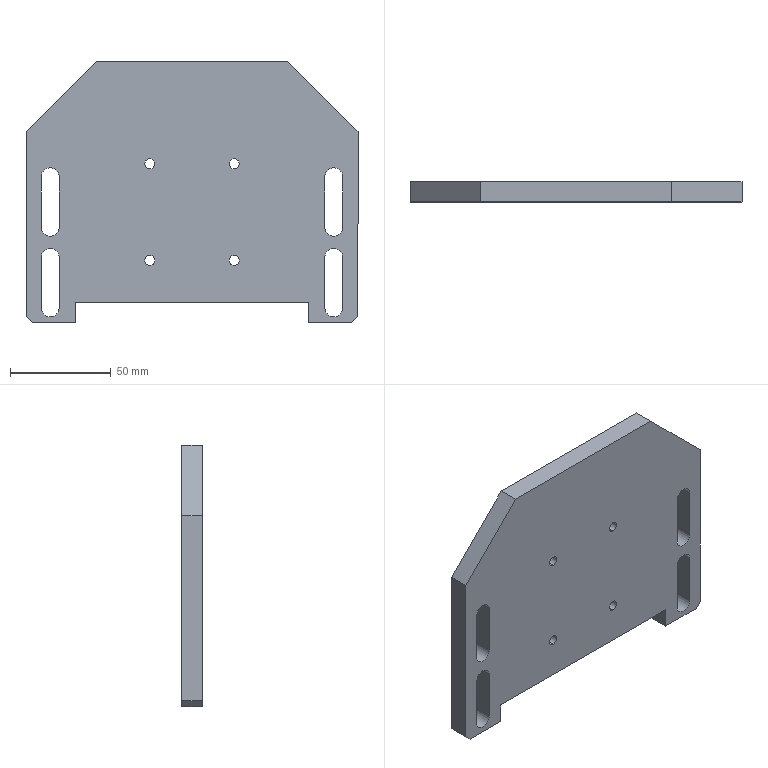Part | SolidWorks | features Chamfer 3, ICE 2, Extrusion 1, HoleWzd 1, MirrorPattern 1 | 1 solid | 42 faces | box 165 x 10 x 130 mm | volume 178230 mm3 | plane 22 | cylinder 20 | commonest cylinder face diameters 9 x12 5 x8
STEP:
#1=CARTESIAN_POINT('',(-66.,0.,7.5));
#2=VERTEX_POINT('',#1);
#3=CARTESIAN_POINT('',(-70.5,0.,12.));
#4=VERTEX_POINT('',#3);
#5=CARTESIAN_POINT('',(-70.5,0.,7.5));
#6=DIRECTION('',(0.,-1.,0.));
#7=DIRECTION('',(0.,0.,1.));
#8=AXIS2_PLACEMENT_3D('',#5,#6,#7);
#9=CIRCLE('',#8,4.5);
#10=EDGE_CURVE('',#2,#4,#9,.T.);
#11=ORIENTED_EDGE('',*,*,#10,.T.);
#12=CARTESIAN_POINT('',(-70.5,10.,12.));
#13=VERTEX_POINT('',#12);
#14=CARTESIAN_POINT('',(-70.5,0.,12.));
#15=DIRECTION('',(0.,1.,0.));
#16=VECTOR('',#15,1000.);
#17=LINE('',#14,#16);
#18=EDGE_CURVE('',#4,#13,#17,.T.);
#19=ORIENTED_EDGE('',*,*,#18,.T.);
#20=CARTESIAN_POINT('',(-66.,10.,7.5));
#21=VERTEX_POINT('',#20);
#22=CARTESIAN_POINT('',(-70.5,10.,7.5));
#23=DIRECTION('',(0.,-1.,0.));
#24=DIRECTION('',(0.,0.,1.));
#25=AXIS2_PLACEMENT_3D('',#22,#23,#24);
#26=CIRCLE('',#25,4.5);
#27=EDGE_CURVE('',#21,#13,#26,.T.);
#28=ORIENTED_EDGE('',*,*,#27,.F.);
#29=CARTESIAN_POINT('',(-66.,0.,7.5));
#30=DIRECTION('',(0.,1.,0.));
#31=VECTOR('',#30,1000.);
#32=LINE('',#29,#31);
#33=EDGE_CURVE('',#2,#21,#32,.T.);
#34=ORIENTED_EDGE('',*,*,#33,.F.);
#35=EDGE_LOOP('',(#11,#19,#28,#34));
#36=FACE_OUTER_BOUND('',#35,.T.);
#37=CARTESIAN_POINT('',(-70.5,0.,7.5));
#38=DIRECTION('',(0.,1.,0.));
#39=DIRECTION('',(0.,0.,1.));
#40=AXIS2_PLACEMENT_3D('',#37,#38,#39);
#41=CYLINDRICAL_SURFACE('',#40,4.5);
#42=ADVANCED_FACE('',(#36),#41,.F.);
#43=CARTESIAN_POINT('',(-66.,0.,-32.5));
#44=VERTEX_POINT('',#43);
#45=CARTESIAN_POINT('',(-70.5,0.,-28.));
#46=VERTEX_POINT('',#45);
#47=CARTESIAN_POINT('',(-70.5,0.,-32.5));
#48=DIRECTION('',(0.,-1.,0.));
#49=DIRECTION('',(0.,0.,1.));
#50=AXIS2_PLACEMENT_3D('',#47,#48,#49);
#51=CIRCLE('',#50,4.5);
#52=EDGE_CURVE('',#44,#46,#51,.T.);
#53=ORIENTED_EDGE('',*,*,#52,.T.);
#54=CARTESIAN_POINT('',(-70.5,10.,-28.));
#55=VERTEX_POINT('',#54);
#56=CARTESIAN_POINT('',(-70.5,0.,-28.));
#57=DIRECTION('',(0.,1.,0.));
#58=VECTOR('',#57,1000.);
#59=LINE('',#56,#58);
#60=EDGE_CURVE('',#46,#55,#59,.T.);
#61=ORIENTED_EDGE('',*,*,#60,.T.);
#62=CARTESIAN_POINT('',(-66.,10.,-32.5));
#63=VERTEX_POINT('',#62);
#64=CARTESIAN_POINT('',(-70.5,10.,-32.5));
#65=DIRECTION('',(0.,-1.,0.));
#66=DIRECTION('',(0.,0.,1.));
#67=AXIS2_PLACEMENT_3D('',#64,#65,#66);
#68=CIRCLE('',#67,4.5);
#69=EDGE_CURVE('',#63,#55,#68,.T.);
#70=ORIENTED_EDGE('',*,*,#69,.F.);
#71=CARTESIAN_POINT('',(-66.,0.,-32.5));
#72=DIRECTION('',(0.,1.,0.));
#73=VECTOR('',#72,1000.);
#74=LINE('',#71,#73);
#75=EDGE_CURVE('',#44,#63,#74,.T.);
#76=ORIENTED_EDGE('',*,*,#75,.F.);
#77=EDGE_LOOP('',(#53,#61,#70,#76));
#78=FACE_OUTER_BOUND('',#77,.T.);
#79=CARTESIAN_POINT('',(-70.5,0.,-32.5));
#80=DIRECTION('',(0.,1.,0.));
#81=DIRECTION('',(0.,0.,1.));
#82=AXIS2_PLACEMENT_3D('',#79,#80,#81);
#83=CYLINDRICAL_SURFACE('',#82,4.5);
#84=ADVANCED_FACE('',(#78),#83,.F.);
#85=CARTESIAN_POINT('',(21.,0.,11.5));
#86=VERTEX_POINT('',#85);
#87=CARTESIAN_POINT('',(21.,0.,16.5));
#88=VERTEX_POINT('',#87);
#89=CARTESIAN_POINT('',(21.,0.,14.));
#90=DIRECTION('',(0.,1.,0.));
#91=DIRECTION('',(0.,0.,1.));
#92=AXIS2_PLACEMENT_3D('',#89,#90,#91);
#93=CIRCLE('',#92,2.5);
#94=EDGE_CURVE('',#86,#88,#93,.T.);
#95=ORIENTED_EDGE('',*,*,#94,.F.);
#96=CARTESIAN_POINT('',(21.,10.,11.5));
#97=VERTEX_POINT('',#96);
#98=CARTESIAN_POINT('',(21.,10.,11.5));
#99=DIRECTION('',(0.,1.,0.));
#100=VECTOR('',#99,1000.);
#101=LINE('',#98,#100);
#102=EDGE_CURVE('',#86,#97,#101,.T.);
#103=ORIENTED_EDGE('',*,*,#102,.T.);
#104=CARTESIAN_POINT('',(21.,10.,16.5));
#105=VERTEX_POINT('',#104);
#106=CARTESIAN_POINT('',(21.,10.,14.));
#107=DIRECTION('',(0.,1.,0.));
#108=DIRECTION('',(0.,0.,1.));
#109=AXIS2_PLACEMENT_3D('',#106,#107,#108);
#110=CIRCLE('',#109,2.5);
#111=EDGE_CURVE('',#97,#105,#110,.T.);
#112=ORIENTED_EDGE('',*,*,#111,.T.);
#113=CARTESIAN_POINT('',(21.,10.,16.5));
#114=DIRECTION('',(0.,1.,0.));
#115=VECTOR('',#114,1000.);
#116=LINE('',#113,#115);
#117=EDGE_CURVE('',#88,#105,#116,.T.);
#118=ORIENTED_EDGE('',*,*,#117,.F.);
#119=EDGE_LOOP('',(#95,#103,#112,#118));
#120=FACE_OUTER_BOUND('',#119,.T.);
#121=CARTESIAN_POINT('',(21.,10.,14.));
#122=DIRECTION('',(0.,1.,0.));
#123=DIRECTION('',(0.,0.,1.));
#124=AXIS2_PLACEMENT_3D('',#121,#122,#123);
#125=CYLINDRICAL_SURFACE('',#124,2.5);
#126=ADVANCED_FACE('',(#120),#125,.F.);
#127=CARTESIAN_POINT('',(21.,0.,-36.5));
#128=VERTEX_POINT('',#127);
#129=CARTESIAN_POINT('',(21.,0.,-31.5));
#130=VERTEX_POINT('',#129);
#131=CARTESIAN_POINT('',(21.,0.,-34.));
#132=DIRECTION('',(0.,1.,0.));
#133=DIRECTION('',(0.,0.,1.));
#134=AXIS2_PLACEMENT_3D('',#131,#132,#133);
#135=CIRCLE('',#134,2.5);
#136=EDGE_CURVE('',#128,#130,#135,.T.);
#137=ORIENTED_EDGE('',*,*,#136,.F.);
#138=CARTESIAN_POINT('',(21.,10.,-36.5));
#139=VERTEX_POINT('',#138);
#140=CARTESIAN_POINT('',(21.,10.,-36.5));
#141=DIRECTION('',(0.,1.,0.));
#142=VECTOR('',#141,1000.);
#143=LINE('',#140,#142);
#144=EDGE_CURVE('',#128,#139,#143,.T.);
#145=ORIENTED_EDGE('',*,*,#144,.T.);
#146=CARTESIAN_POINT('',(21.,10.,-31.5));
#147=VERTEX_POINT('',#146);
#148=CARTESIAN_POINT('',(21.,10.,-34.));
#149=DIRECTION('',(0.,1.,0.));
#150=DIRECTION('',(0.,0.,1.));
#151=AXIS2_PLACEMENT_3D('',#148,#149,#150);
#152=CIRCLE('',#151,2.5);
#153=EDGE_CURVE('',#139,#147,#152,.T.);
#154=ORIENTED_EDGE('',*,*,#153,.T.);
#155=CARTESIAN_POINT('',(21.,10.,-31.5));
#156=DIRECTION('',(0.,1.,0.));
#157=VECTOR('',#156,1000.);
#158=LINE('',#155,#157);
#159=EDGE_CURVE('',#130,#147,#158,.T.);
#160=ORIENTED_EDGE('',*,*,#159,.F.);
#161=EDGE_LOOP('',(#137,#145,#154,#160));
#162=FACE_OUTER_BOUND('',#161,.T.);
#163=CARTESIAN_POINT('',(21.,10.,-34.));
#164=DIRECTION('',(0.,1.,0.));
#165=DIRECTION('',(0.,0.,1.));
#166=AXIS2_PLACEMENT_3D('',#163,#164,#165);
#167=CYLINDRICAL_SURFACE('',#166,2.5);
#168=ADVANCED_FACE('',(#162),#167,.F.);
#169=CARTESIAN_POINT('',(-21.,0.,-36.5));
#170=VERTEX_POINT('',#169);
#171=CARTESIAN_POINT('',(-21.,0.,-31.5));
#172=VERTEX_POINT('',#171);
#173=CARTESIAN_POINT('',(-21.,0.,-34.));
#174=DIRECTION('',(0.,1.,0.));
#175=DIRECTION('',(0.,0.,1.));
#176=AXIS2_PLACEMENT_3D('',#173,#174,#175);
#177=CIRCLE('',#176,2.5);
#178=EDGE_CURVE('',#170,#172,#177,.T.);
#179=ORIENTED_EDGE('',*,*,#178,.F.);
#180=CARTESIAN_POINT('',(-21.,10.,-36.5));
#181=VERTEX_POINT('',#180);
#182=CARTESIAN_POINT('',(-21.,10.,-36.5));
#183=DIRECTION('',(0.,1.,0.));
#184=VECTOR('',#183,1000.);
#185=LINE('',#182,#184);
#186=EDGE_CURVE('',#170,#181,#185,.T.);
#187=ORIENTED_EDGE('',*,*,#186,.T.);
#188=CARTESIAN_POINT('',(-21.,10.,-31.5));
#189=VERTEX_POINT('',#188);
#190=CARTESIAN_POINT('',(-21.,10.,-34.));
#191=DIRECTION('',(0.,1.,0.));
#192=DIRECTION('',(0.,0.,1.));
#193=AXIS2_PLACEMENT_3D('',#190,#191,#192);
#194=CIRCLE('',#193,2.5);
#195=EDGE_CURVE('',#181,#189,#194,.T.);
#196=ORIENTED_EDGE('',*,*,#195,.T.);
#197=CARTESIAN_POINT('',(-21.,10.,-31.5));
#198=DIRECTION('',(0.,1.,0.));
#199=VECTOR('',#198,1000.);
#200=LINE('',#197,#199);
#201=EDGE_CURVE('',#172,#189,#200,.T.);
#202=ORIENTED_EDGE('',*,*,#201,.F.);
#203=EDGE_LOOP('',(#179,#187,#196,#202));
#204=FACE_OUTER_BOUND('',#203,.T.);
#205=CARTESIAN_POINT('',(-21.,10.,-34.));
#206=DIRECTION('',(0.,1.,0.));
#207=DIRECTION('',(0.,0.,1.));
#208=AXIS2_PLACEMENT_3D('',#205,#206,#207);
#209=CYLINDRICAL_SURFACE('',#208,2.5);
#210=ADVANCED_FACE('',(#204),#209,.F.);
#211=CARTESIAN_POINT('',(-21.,0.,11.5));
#212=VERTEX_POINT('',#211);
#213=CARTESIAN_POINT('',(-21.,0.,16.5));
#214=VERTEX_POINT('',#213);
#215=CARTESIAN_POINT('',(-21.,0.,14.));
#216=DIRECTION('',(0.,1.,0.));
#217=DIRECTION('',(0.,0.,1.));
#218=AXIS2_PLACEMENT_3D('',#215,#216,#217);
#219=CIRCLE('',#218,2.5);
#220=EDGE_CURVE('',#212,#214,#219,.T.);
#221=ORIENTED_EDGE('',*,*,#220,.F.);
#222=CARTESIAN_POINT('',(-21.,10.,11.5));
#223=VERTEX_POINT('',#222);
#224=CARTESIAN_POINT('',(-21.,10.,11.5));
#225=DIRECTION('',(0.,1.,0.));
#226=VECTOR('',#225,1000.);
#227=LINE('',#224,#226);
#228=EDGE_CURVE('',#212,#223,#227,.T.);
#229=ORIENTED_EDGE('',*,*,#228,.T.);
#230=CARTESIAN_POINT('',(-21.,10.,16.5));
#231=VERTEX_POINT('',#230);
#232=CARTESIAN_POINT('',(-21.,10.,14.));
#233=DIRECTION('',(0.,1.,0.));
#234=DIRECTION('',(0.,0.,1.));
#235=AXIS2_PLACEMENT_3D('',#232,#233,#234);
#236=CIRCLE('',#235,2.5);
#237=EDGE_CURVE('',#223,#231,#236,.T.);
#238=ORIENTED_EDGE('',*,*,#237,.T.);
#239=CARTESIAN_POINT('',(-21.,10.,16.5));
#240=DIRECTION('',(0.,1.,0.));
#241=VECTOR('',#240,1000.);
#242=LINE('',#239,#241);
#243=EDGE_CURVE('',#214,#231,#242,.T.);
#244=ORIENTED_EDGE('',*,*,#243,.F.);
#245=EDGE_LOOP('',(#221,#229,#238,#244));
#246=FACE_OUTER_BOUND('',#245,.T.);
#247=CARTESIAN_POINT('',(-21.,10.,14.));
#248=DIRECTION('',(0.,1.,0.));
#249=DIRECTION('',(0.,0.,1.));
#250=AXIS2_PLACEMENT_3D('',#247,#248,#249);
#251=CYLINDRICAL_SURFACE('',#250,2.5);
#252=ADVANCED_FACE('',(#246),#251,.F.);
#253=CARTESIAN_POINT('',(70.5,0.,12.));
#254=VERTEX_POINT('',#253);
#255=CARTESIAN_POINT('',(75.,0.,7.5));
#256=VERTEX_POINT('',#255);
#257=CARTESIAN_POINT('',(70.5,0.,7.5));
#258=DIRECTION('',(0.,1.,0.));
#259=DIRECTION('',(0.,0.,1.));
#260=AXIS2_PLACEMENT_3D('',#257,#258,#259);
#261=CIRCLE('',#260,4.5);
#262=EDGE_CURVE('',#254,#256,#261,.T.);
#263=ORIENTED_EDGE('',*,*,#262,.F.);
#264=CARTESIAN_POINT('',(70.5,10.,12.));
#265=VERTEX_POINT('',#264);
#266=CARTESIAN_POINT('',(70.5,0.,12.));
#267=DIRECTION('',(0.,1.,0.));
#268=VECTOR('',#267,1000.);
#269=LINE('',#266,#268);
#270=EDGE_CURVE('',#254,#265,#269,.T.);
#271=ORIENTED_EDGE('',*,*,#270,.T.);
#272=CARTESIAN_POINT('',(75.,10.,7.5));
#273=VERTEX_POINT('',#272);
#274=CARTESIAN_POINT('',(70.5,10.,7.5));
#275=DIRECTION('',(0.,1.,0.));
#276=DIRECTION('',(0.,0.,1.));
#277=AXIS2_PLACEMENT_3D('',#274,#275,#276);
#278=CIRCLE('',#277,4.5);
#279=EDGE_CURVE('',#265,#273,#278,.T.);
#280=ORIENTED_EDGE('',*,*,#279,.T.);
#281=CARTESIAN_POINT('',(75.,0.,7.5));
#282=DIRECTION('',(0.,1.,0.));
#283=VECTOR('',#282,1000.);
#284=LINE('',#281,#283);
#285=EDGE_CURVE('',#256,#273,#284,.T.);
#286=ORIENTED_EDGE('',*,*,#285,.F.);
#287=EDGE_LOOP('',(#263,#271,#280,#286));
#288=FACE_OUTER_BOUND('',#287,.T.);
#289=CARTESIAN_POINT('',(70.5,0.,7.5));
#290=DIRECTION('',(0.,1.,0.));
#291=DIRECTION('',(0.,0.,1.));
#292=AXIS2_PLACEMENT_3D('',#289,#290,#291);
#293=CYLINDRICAL_SURFACE('',#292,4.5);
#294=ADVANCED_FACE('',(#288),#293,.F.);
#295=CARTESIAN_POINT('',(70.5,0.,-28.));
#296=VERTEX_POINT('',#295);
#297=CARTESIAN_POINT('',(75.,0.,-32.5));
#298=VERTEX_POINT('',#297);
#299=CARTESIAN_POINT('',(70.5,0.,-32.5));
#300=DIRECTION('',(0.,1.,0.));
#301=DIRECTION('',(0.,0.,1.));
#302=AXIS2_PLACEMENT_3D('',#299,#300,#301);
#303=CIRCLE('',#302,4.5);
#304=EDGE_CURVE('',#296,#298,#303,.T.);
#305=ORIENTED_EDGE('',*,*,#304,.F.);
#306=CARTESIAN_POINT('',(70.5,10.,-28.));
#307=VERTEX_POINT('',#306);
#308=CARTESIAN_POINT('',(70.5,0.,-28.));
#309=DIRECTION('',(0.,1.,0.));
#310=VECTOR('',#309,1000.);
#311=LINE('',#308,#310);
#312=EDGE_CURVE('',#296,#307,#311,.T.);
#313=ORIENTED_EDGE('',*,*,#312,.T.);
#314=CARTESIAN_POINT('',(75.,10.,-32.5));
#315=VERTEX_POINT('',#314);
#316=CARTESIAN_POINT('',(70.5,10.,-32.5));
#317=DIRECTION('',(0.,1.,0.));
#318=DIRECTION('',(0.,0.,1.));
#319=AXIS2_PLACEMENT_3D('',#316,#317,#318);
#320=CIRCLE('',#319,4.5);
#321=EDGE_CURVE('',#307,#315,#320,.T.);
#322=ORIENTED_EDGE('',*,*,#321,.T.);
#323=CARTESIAN_POINT('',(75.,0.,-32.5));
#324=DIRECTION('',(0.,1.,0.));
#325=VECTOR('',#324,1000.);
#326=LINE('',#323,#325);
#327=EDGE_CURVE('',#298,#315,#326,.T.);
#328=ORIENTED_EDGE('',*,*,#327,.F.);
#329=EDGE_LOOP('',(#305,#313,#322,#328));
#330=FACE_OUTER_BOUND('',#329,.T.);
#331=CARTESIAN_POINT('',(70.5,0.,-32.5));
#332=DIRECTION('',(0.,1.,0.));
#333=DIRECTION('',(0.,0.,1.));
#334=AXIS2_PLACEMENT_3D('',#331,#332,#333);
#335=CYLINDRICAL_SURFACE('',#334,4.5);
#336=ADVANCED_FACE('',(#330),#335,.F.);
#337=CARTESIAN_POINT('',(-75.,10.,-32.5));
#338=VERTEX_POINT('',#337);
#339=CARTESIAN_POINT('',(-75.,10.,-57.5));
#340=VERTEX_POINT('',#339);
#341=CARTESIAN_POINT('',(-75.,10.,-57.5));
#342=DIRECTION('',(0.,0.,-1.));
#343=VECTOR('',#342,1000.);
#344=LINE('',#341,#343);
#345=EDGE_CURVE('',#338,#340,#344,.T.);
#346=ORIENTED_EDGE('',*,*,#345,.T.);
#347=CARTESIAN_POINT('',(-66.,10.,-57.5));
#348=VERTEX_POINT('',#347);
#349=CARTESIAN_POINT('',(-70.5,10.,-57.5));
#350=DIRECTION('',(0.,-1.,0.));
#351=DIRECTION('',(0.,0.,1.));
#352=AXIS2_PLACEMENT_3D('',#349,#350,#351);
#353=CIRCLE('',#352,4.5);
#354=EDGE_CURVE('',#340,#348,#353,.T.);
#355=ORIENTED_EDGE('',*,*,#354,.T.);
#356=CARTESIAN_POINT('',(-66.,10.,-57.5));
#357=DIRECTION('',(0.,0.,1.));
#358=VECTOR('',#357,1000.);
#359=LINE('',#356,#358);
#360=EDGE_CURVE('',#348,#63,#359,.T.);
#361=ORIENTED_EDGE('',*,*,#360,.T.);
#362=ORIENTED_EDGE('',*,*,#69,.T.);
#363=CARTESIAN_POINT('',(-70.5,10.,-32.5));
#364=DIRECTION('',(0.,-1.,0.));
#365=DIRECTION('',(0.,0.,1.));
#366=AXIS2_PLACEMENT_3D('',#363,#364,#365);
#367=CIRCLE('',#366,4.5);
#368=EDGE_CURVE('',#55,#338,#367,.T.);
#369=ORIENTED_EDGE('',*,*,#368,.T.);
#370=EDGE_LOOP('',(#346,#355,#361,#362,#369));
#371=FACE_BOUND('',#370,.T.);
#372=CARTESIAN_POINT('',(21.,10.,14.));
#373=DIRECTION('',(0.,1.,0.));
#374=DIRECTION('',(0.,0.,1.));
#375=AXIS2_PLACEMENT_3D('',#372,#373,#374);
#376=CIRCLE('',#375,2.5);
#377=EDGE_CURVE('',#105,#97,#376,.T.);
#378=ORIENTED_EDGE('',*,*,#377,.F.);
#379=ORIENTED_EDGE('',*,*,#111,.F.);
#380=EDGE_LOOP('',(#378,#379));
#381=FACE_BOUND('',#380,.T.);
#382=CARTESIAN_POINT('',(21.,10.,-34.));
#383=DIRECTION('',(0.,1.,0.));
#384=DIRECTION('',(0.,0.,1.));
#385=AXIS2_PLACEMENT_3D('',#382,#383,#384);
#386=CIRCLE('',#385,2.5);
#387=EDGE_CURVE('',#147,#139,#386,.T.);
#388=ORIENTED_EDGE('',*,*,#387,.F.);
#389=ORIENTED_EDGE('',*,*,#153,.F.);
#390=EDGE_LOOP('',(#388,#389));
#391=FACE_BOUND('',#390,.T.);
#392=CARTESIAN_POINT('',(-21.,10.,-34.));
#393=DIRECTION('',(0.,1.,0.));
#394=DIRECTION('',(0.,0.,1.));
#395=AXIS2_PLACEMENT_3D('',#392,#393,#394);
#396=CIRCLE('',#395,2.5);
#397=EDGE_CURVE('',#189,#181,#396,.T.);
#398=ORIENTED_EDGE('',*,*,#397,.F.);
#399=ORIENTED_EDGE('',*,*,#195,.F.);
#400=EDGE_LOOP('',(#398,#399));
#401=FACE_BOUND('',#400,.T.);
#402=CARTESIAN_POINT('',(-21.,10.,14.));
#403=DIRECTION('',(0.,1.,0.));
#404=DIRECTION('',(0.,0.,1.));
#405=AXIS2_PLACEMENT_3D('',#402,#403,#404);
#406=CIRCLE('',#405,2.5);
#407=EDGE_CURVE('',#231,#223,#406,.T.);
#408=ORIENTED_EDGE('',*,*,#407,.F.);
#409=ORIENTED_EDGE('',*,*,#237,.F.);
#410=EDGE_LOOP('',(#408,#409));
#411=FACE_BOUND('',#410,.T.);
#412=CARTESIAN_POINT('',(75.,10.,-17.5));
#413=VERTEX_POINT('',#412);
#414=CARTESIAN_POINT('',(66.,10.,-17.5));
#415=VERTEX_POINT('',#414);
#416=CARTESIAN_POINT('',(70.5,10.,-17.5));
#417=DIRECTION('',(0.,1.,0.));
#418=DIRECTION('',(0.,0.,1.));
#419=AXIS2_PLACEMENT_3D('',#416,#417,#418);
#420=CIRCLE('',#419,4.5);
#421=EDGE_CURVE('',#413,#415,#420,.T.);
#422=ORIENTED_EDGE('',*,*,#421,.F.);
#423=CARTESIAN_POINT('',(75.,10.,-17.5));
#424=DIRECTION('',(0.,0.,-1.));
#425=VECTOR('',#424,1000.);
#426=LINE('',#423,#425);
#427=EDGE_CURVE('',#273,#413,#426,.T.);
#428=ORIENTED_EDGE('',*,*,#427,.F.);
#429=ORIENTED_EDGE('',*,*,#279,.F.);
#430=CARTESIAN_POINT('',(66.,10.,7.5));
#431=VERTEX_POINT('',#430);
#432=CARTESIAN_POINT('',(70.5,10.,7.5));
#433=DIRECTION('',(0.,1.,0.));
#434=DIRECTION('',(0.,0.,1.));
#435=AXIS2_PLACEMENT_3D('',#432,#433,#434);
#436=CIRCLE('',#435,4.5);
#437=EDGE_CURVE('',#431,#265,#436,.T.);
#438=ORIENTED_EDGE('',*,*,#437,.F.);
#439=CARTESIAN_POINT('',(66.,10.,-17.5));
#440=DIRECTION('',(0.,0.,1.));
#441=VECTOR('',#440,1000.);
#442=LINE('',#439,#441);
#443=EDGE_CURVE('',#415,#431,#442,.T.);
#444=ORIENTED_EDGE('',*,*,#443,.F.);
#445=EDGE_LOOP('',(#422,#428,#429,#438,#444));
#446=FACE_BOUND('',#445,.T.);
#447=CARTESIAN_POINT('',(75.,10.,-57.5));
#448=VERTEX_POINT('',#447);
#449=CARTESIAN_POINT('',(66.,10.,-57.5));
#450=VERTEX_POINT('',#449);
#451=CARTESIAN_POINT('',(70.5,10.,-57.5));
#452=DIRECTION('',(0.,1.,0.));
#453=DIRECTION('',(0.,0.,1.));
#454=AXIS2_PLACEMENT_3D('',#451,#452,#453);
#455=CIRCLE('',#454,4.5);
#456=EDGE_CURVE('',#448,#450,#455,.T.);
#457=ORIENTED_EDGE('',*,*,#456,.F.);
#458=CARTESIAN_POINT('',(75.,10.,-57.5));
#459=DIRECTION('',(0.,0.,-1.));
#460=VECTOR('',#459,1000.);
#461=LINE('',#458,#460);
#462=EDGE_CURVE('',#315,#448,#461,.T.);
#463=ORIENTED_EDGE('',*,*,#462,.F.);
#464=ORIENTED_EDGE('',*,*,#321,.F.);
#465=CARTESIAN_POINT('',(66.,10.,-32.5));
#466=VERTEX_POINT('',#465);
#467=CARTESIAN_POINT('',(70.5,10.,-32.5));
#468=DIRECTION('',(0.,1.,0.));
#469=DIRECTION('',(0.,0.,1.));
#470=AXIS2_PLACEMENT_3D('',#467,#468,#469);
#471=CIRCLE('',#470,4.5);
#472=EDGE_CURVE('',#466,#307,#471,.T.);
#473=ORIENTED_EDGE('',*,*,#472,.F.);
#474=CARTESIAN_POINT('',(66.,10.,-57.5));
#475=DIRECTION('',(0.,0.,1.));
#476=VECTOR('',#475,1000.);
#477=LINE('',#474,#476);
#478=EDGE_CURVE('',#450,#466,#477,.T.);
#479=ORIENTED_EDGE('',*,*,#478,.F.);
#480=EDGE_LOOP('',(#457,#463,#464,#473,#479));
#481=FACE_BOUND('',#480,.T.);
#482=CARTESIAN_POINT('',(82.5,10.,30.));
#483=VERTEX_POINT('',#482);
#484=CARTESIAN_POINT('',(82.5,10.,-62.));
#485=VERTEX_POINT('',#484);
#486=CARTESIAN_POINT('',(82.5,10.,-65.));
#487=DIRECTION('',(0.,0.,-1.));
#488=VECTOR('',#487,1000.);
#489=LINE('',#486,#488);
#490=EDGE_CURVE('',#483,#485,#489,.T.);
#491=ORIENTED_EDGE('',*,*,#490,.T.);
#492=CARTESIAN_POINT('',(79.5,10.,-65.));
#493=VERTEX_POINT('',#492);
#494=CARTESIAN_POINT('',(72.25,10.,-72.25));
#495=DIRECTION('',(-0.7071,0.,-0.7071));
#496=VECTOR('',#495,1000.);
#497=LINE('',#494,#496);
#498=EDGE_CURVE('',#485,#493,#497,.T.);
#499=ORIENTED_EDGE('',*,*,#498,.T.);
#500=CARTESIAN_POINT('',(58.,10.,-65.));
#501=VERTEX_POINT('',#500);
#502=CARTESIAN_POINT('',(-82.5,10.,-65.));
#503=DIRECTION('',(-1.,0.,0.));
#504=VECTOR('',#503,1000.);
#505=LINE('',#502,#504);
#506=EDGE_CURVE('',#493,#501,#505,.T.);
#507=ORIENTED_EDGE('',*,*,#506,.T.);
#508=CARTESIAN_POINT('',(58.,10.,-55.));
#509=VERTEX_POINT('',#508);
#510=CARTESIAN_POINT('',(58.,10.,-65.));
#511=DIRECTION('',(0.,0.,-1.));
#512=VECTOR('',#511,1000.);
#513=LINE('',#510,#512);
#514=EDGE_CURVE('',#509,#501,#513,.T.);
#515=ORIENTED_EDGE('',*,*,#514,.F.);
#516=CARTESIAN_POINT('',(-58.,10.,-55.));
#517=VERTEX_POINT('',#516);
#518=CARTESIAN_POINT('',(-58.,10.,-55.));
#519=DIRECTION('',(1.,0.,0.));
#520=VECTOR('',#519,1000.);
#521=LINE('',#518,#520);
#522=EDGE_CURVE('',#517,#509,#521,.T.);
#523=ORIENTED_EDGE('',*,*,#522,.F.);
#524=CARTESIAN_POINT('',(-58.,10.,-65.));
#525=VERTEX_POINT('',#524);
#526=CARTESIAN_POINT('',(-58.,10.,-65.));
#527=DIRECTION('',(0.,0.,1.));
#528=VECTOR('',#527,1000.);
#529=LINE('',#526,#528);
#530=EDGE_CURVE('',#525,#517,#529,.T.);
#531=ORIENTED_EDGE('',*,*,#530,.F.);
#532=CARTESIAN_POINT('',(-79.5,10.,-65.));
#533=VERTEX_POINT('',#532);
#534=CARTESIAN_POINT('',(-82.5,10.,-65.));
#535=DIRECTION('',(-1.,0.,0.));
#536=VECTOR('',#535,1000.);
#537=LINE('',#534,#536);
#538=EDGE_CURVE('',#525,#533,#537,.T.);
#539=ORIENTED_EDGE('',*,*,#538,.T.);
#540=CARTESIAN_POINT('',(-82.5,10.,-62.));
#541=VERTEX_POINT('',#540);
#542=CARTESIAN_POINT('',(-72.25,10.,-72.25));
#543=DIRECTION('',(-0.7071,0.,0.7071));
#544=VECTOR('',#543,1000.);
#545=LINE('',#542,#544);
#546=EDGE_CURVE('',#533,#541,#545,.T.);
#547=ORIENTED_EDGE('',*,*,#546,.T.);
#548=CARTESIAN_POINT('',(-82.5,10.,30.));
#549=VERTEX_POINT('',#548);
#550=CARTESIAN_POINT('',(-82.5,10.,-65.));
#551=DIRECTION('',(0.,0.,1.));
#552=VECTOR('',#551,1000.);
#553=LINE('',#550,#552);
#554=EDGE_CURVE('',#541,#549,#553,.T.);
#555=ORIENTED_EDGE('',*,*,#554,.T.);
#556=CARTESIAN_POINT('',(-47.5,10.,65.));
#557=VERTEX_POINT('',#556);
#558=CARTESIAN_POINT('',(-56.25,10.,56.25));
#559=DIRECTION('',(0.7071,0.,0.7071));
#560=VECTOR('',#559,1000.);
#561=LINE('',#558,#560);
#562=EDGE_CURVE('',#549,#557,#561,.T.);
#563=ORIENTED_EDGE('',*,*,#562,.T.);
#564=CARTESIAN_POINT('',(47.5,10.,65.));
#565=VERTEX_POINT('',#564);
#566=CARTESIAN_POINT('',(-82.5,10.,65.));
#567=DIRECTION('',(1.,0.,0.));
#568=VECTOR('',#567,1000.);
#569=LINE('',#566,#568);
#570=EDGE_CURVE('',#557,#565,#569,.T.);
#571=ORIENTED_EDGE('',*,*,#570,.T.);
#572=CARTESIAN_POINT('',(56.25,10.,56.25));
#573=DIRECTION('',(0.7071,0.,-0.7071));
#574=VECTOR('',#573,1000.);
#575=LINE('',#572,#574);
#576=EDGE_CURVE('',#565,#483,#575,.T.);
#577=ORIENTED_EDGE('',*,*,#576,.T.);
#578=EDGE_LOOP('',(#491,#499,#507,#515,#523,#531,#539,#547,#555,#563,#571,#577));
#579=FACE_OUTER_BOUND('',#578,.T.);
#580=CARTESIAN_POINT('',(-75.,10.,7.5));
#581=VERTEX_POINT('',#580);
#582=CARTESIAN_POINT('',(-75.,10.,-17.5));
#583=VERTEX_POINT('',#582);
#584=CARTESIAN_POINT('',(-75.,10.,-17.5));
#585=DIRECTION('',(0.,0.,-1.));
#586=VECTOR('',#585,1000.);
#587=LINE('',#584,#586);
#588=EDGE_CURVE('',#581,#583,#587,.T.);
#589=ORIENTED_EDGE('',*,*,#588,.T.);
#590=CARTESIAN_POINT('',(-66.,10.,-17.5));
#591=VERTEX_POINT('',#590);
#592=CARTESIAN_POINT('',(-70.5,10.,-17.5));
#593=DIRECTION('',(0.,-1.,0.));
#594=DIRECTION('',(0.,0.,1.));
#595=AXIS2_PLACEMENT_3D('',#592,#593,#594);
#596=CIRCLE('',#595,4.5);
#597=EDGE_CURVE('',#583,#591,#596,.T.);
#598=ORIENTED_EDGE('',*,*,#597,.T.);
#599=CARTESIAN_POINT('',(-66.,10.,-17.5));
#600=DIRECTION('',(0.,0.,1.));
#601=VECTOR('',#600,1000.);
#602=LINE('',#599,#601);
#603=EDGE_CURVE('',#591,#21,#602,.T.);
#604=ORIENTED_EDGE('',*,*,#603,.T.);
#605=ORIENTED_EDGE('',*,*,#27,.T.);
#606=CARTESIAN_POINT('',(-70.5,10.,7.5));
#607=DIRECTION('',(0.,-1.,0.));
#608=DIRECTION('',(0.,0.,1.));
#609=AXIS2_PLACEMENT_3D('',#606,#607,#608);
#610=CIRCLE('',#609,4.5);
#611=EDGE_CURVE('',#13,#581,#610,.T.);
#612=ORIENTED_EDGE('',*,*,#611,.T.);
#613=EDGE_LOOP('',(#589,#598,#604,#605,#612));
#614=FACE_BOUND('',#613,.T.);
#615=CARTESIAN_POINT('',(0.,10.,0.));
#616=DIRECTION('',(0.,1.,0.));
#617=DIRECTION('',(0.,0.,1.));
#618=AXIS2_PLACEMENT_3D('',#615,#616,#617);
#619=PLANE('',#618);
#620=ADVANCED_FACE('',(#371,#381,#391,#401,#411,#446,#481,#579,#614),#619,.T.);
#621=CARTESIAN_POINT('',(-75.,0.,-57.5));
#622=VERTEX_POINT('',#621);
#623=CARTESIAN_POINT('',(-66.,0.,-57.5));
#624=VERTEX_POINT('',#623);
#625=CARTESIAN_POINT('',(-70.5,0.,-57.5));
#626=DIRECTION('',(0.,-1.,0.));
#627=DIRECTION('',(0.,0.,1.));
#628=AXIS2_PLACEMENT_3D('',#625,#626,#627);
#629=CIRCLE('',#628,4.5);
#630=EDGE_CURVE('',#622,#624,#629,.T.);
#631=ORIENTED_EDGE('',*,*,#630,.F.);
#632=CARTESIAN_POINT('',(-75.,0.,-32.5));
#633=VERTEX_POINT('',#632);
#634=CARTESIAN_POINT('',(-75.,0.,-57.5));
#635=DIRECTION('',(0.,0.,-1.));
#636=VECTOR('',#635,1000.);
#637=LINE('',#634,#636);
#638=EDGE_CURVE('',#633,#622,#637,.T.);
#639=ORIENTED_EDGE('',*,*,#638,.F.);
#640=CARTESIAN_POINT('',(-70.5,0.,-32.5));
#641=DIRECTION('',(0.,-1.,0.));
#642=DIRECTION('',(0.,0.,1.));
#643=AXIS2_PLACEMENT_3D('',#640,#641,#642);
#644=CIRCLE('',#643,4.5);
#645=EDGE_CURVE('',#46,#633,#644,.T.);
#646=ORIENTED_EDGE('',*,*,#645,.F.);
#647=ORIENTED_EDGE('',*,*,#52,.F.);
#648=CARTESIAN_POINT('',(-66.,0.,-57.5));
#649=DIRECTION('',(0.,0.,1.));
#650=VECTOR('',#649,1000.);
#651=LINE('',#648,#650);
#652=EDGE_CURVE('',#624,#44,#651,.T.);
#653=ORIENTED_EDGE('',*,*,#652,.F.);
#654=EDGE_LOOP('',(#631,#639,#646,#647,#653));
#655=FACE_BOUND('',#654,.T.);
#656=CARTESIAN_POINT('',(21.,0.,14.));
#657=DIRECTION('',(0.,1.,0.));
#658=DIRECTION('',(0.,0.,1.));
#659=AXIS2_PLACEMENT_3D('',#656,#657,#658);
#660=CIRCLE('',#659,2.5);
#661=EDGE_CURVE('',#88,#86,#660,.T.);
#662=ORIENTED_EDGE('',*,*,#661,.T.);
#663=ORIENTED_EDGE('',*,*,#94,.T.);
#664=EDGE_LOOP('',(#662,#663));
#665=FACE_BOUND('',#664,.T.);
#666=CARTESIAN_POINT('',(21.,0.,-34.));
#667=DIRECTION('',(0.,1.,0.));
#668=DIRECTION('',(0.,0.,1.));
#669=AXIS2_PLACEMENT_3D('',#666,#667,#668);
#670=CIRCLE('',#669,2.5);
#671=EDGE_CURVE('',#130,#128,#670,.T.);
#672=ORIENTED_EDGE('',*,*,#671,.T.);
#673=ORIENTED_EDGE('',*,*,#136,.T.);
#674=EDGE_LOOP('',(#672,#673));
#675=FACE_BOUND('',#674,.T.);
#676=CARTESIAN_POINT('',(-21.,0.,-34.));
#677=DIRECTION('',(0.,1.,0.));
#678=DIRECTION('',(0.,0.,1.));
#679=AXIS2_PLACEMENT_3D('',#676,#677,#678);
#680=CIRCLE('',#679,2.5);
#681=EDGE_CURVE('',#172,#170,#680,.T.);
#682=ORIENTED_EDGE('',*,*,#681,.T.);
#683=ORIENTED_EDGE('',*,*,#178,.T.);
#684=EDGE_LOOP('',(#682,#683));
#685=FACE_BOUND('',#684,.T.);
#686=CARTESIAN_POINT('',(-21.,0.,14.));
#687=DIRECTION('',(0.,1.,0.));
#688=DIRECTION('',(0.,0.,1.));
#689=AXIS2_PLACEMENT_3D('',#686,#687,#688);
#690=CIRCLE('',#689,2.5);
#691=EDGE_CURVE('',#214,#212,#690,.T.);
#692=ORIENTED_EDGE('',*,*,#691,.T.);
#693=ORIENTED_EDGE('',*,*,#220,.T.);
#694=EDGE_LOOP('',(#692,#693));
#695=FACE_BOUND('',#694,.T.);
#696=CARTESIAN_POINT('',(75.,0.,-17.5));
#697=VERTEX_POINT('',#696);
#698=CARTESIAN_POINT('',(75.,0.,-17.5));
#699=DIRECTION('',(0.,0.,-1.));
#700=VECTOR('',#699,1000.);
#701=LINE('',#698,#700);
#702=EDGE_CURVE('',#256,#697,#701,.T.);
#703=ORIENTED_EDGE('',*,*,#702,.T.);
#704=CARTESIAN_POINT('',(66.,0.,-17.5));
#705=VERTEX_POINT('',#704);
#706=CARTESIAN_POINT('',(70.5,0.,-17.5));
#707=DIRECTION('',(0.,1.,0.));
#708=DIRECTION('',(0.,0.,1.));
#709=AXIS2_PLACEMENT_3D('',#706,#707,#708);
#710=CIRCLE('',#709,4.5);
#711=EDGE_CURVE('',#697,#705,#710,.T.);
#712=ORIENTED_EDGE('',*,*,#711,.T.);
#713=CARTESIAN_POINT('',(66.,0.,7.5));
#714=VERTEX_POINT('',#713);
#715=CARTESIAN_POINT('',(66.,0.,-17.5));
#716=DIRECTION('',(0.,0.,1.));
#717=VECTOR('',#716,1000.);
#718=LINE('',#715,#717);
#719=EDGE_CURVE('',#705,#714,#718,.T.);
#720=ORIENTED_EDGE('',*,*,#719,.T.);
#721=CARTESIAN_POINT('',(70.5,0.,7.5));
#722=DIRECTION('',(0.,1.,0.));
#723=DIRECTION('',(0.,0.,1.));
#724=AXIS2_PLACEMENT_3D('',#721,#722,#723);
#725=CIRCLE('',#724,4.5);
#726=EDGE_CURVE('',#714,#254,#725,.T.);
#727=ORIENTED_EDGE('',*,*,#726,.T.);
#728=ORIENTED_EDGE('',*,*,#262,.T.);
#729=EDGE_LOOP('',(#703,#712,#720,#727,#728));
#730=FACE_BOUND('',#729,.T.);
#731=CARTESIAN_POINT('',(75.,0.,-57.5));
#732=VERTEX_POINT('',#731);
#733=CARTESIAN_POINT('',(75.,0.,-57.5));
#734=DIRECTION('',(0.,0.,-1.));
#735=VECTOR('',#734,1000.);
#736=LINE('',#733,#735);
#737=EDGE_CURVE('',#298,#732,#736,.T.);
#738=ORIENTED_EDGE('',*,*,#737,.T.);
#739=CARTESIAN_POINT('',(66.,0.,-57.5));
#740=VERTEX_POINT('',#739);
#741=CARTESIAN_POINT('',(70.5,0.,-57.5));
#742=DIRECTION('',(0.,1.,0.));
#743=DIRECTION('',(0.,0.,1.));
#744=AXIS2_PLACEMENT_3D('',#741,#742,#743);
#745=CIRCLE('',#744,4.5);
#746=EDGE_CURVE('',#732,#740,#745,.T.);
#747=ORIENTED_EDGE('',*,*,#746,.T.);
#748=CARTESIAN_POINT('',(66.,0.,-32.5));
#749=VERTEX_POINT('',#748);
#750=CARTESIAN_POINT('',(66.,0.,-57.5));
#751=DIRECTION('',(0.,0.,1.));
#752=VECTOR('',#751,1000.);
#753=LINE('',#750,#752);
#754=EDGE_CURVE('',#740,#749,#753,.T.);
#755=ORIENTED_EDGE('',*,*,#754,.T.);
#756=CARTESIAN_POINT('',(70.5,0.,-32.5));
#757=DIRECTION('',(0.,1.,0.));
#758=DIRECTION('',(0.,0.,1.));
#759=AXIS2_PLACEMENT_3D('',#756,#757,#758);
#760=CIRCLE('',#759,4.5);
#761=EDGE_CURVE('',#749,#296,#760,.T.);
#762=ORIENTED_EDGE('',*,*,#761,.T.);
#763=ORIENTED_EDGE('',*,*,#304,.T.);
#764=EDGE_LOOP('',(#738,#747,#755,#762,#763));
#765=FACE_BOUND('',#764,.T.);
#766=CARTESIAN_POINT('',(79.5,0.,-65.));
#767=VERTEX_POINT('',#766);
#768=CARTESIAN_POINT('',(58.,0.,-65.));
#769=VERTEX_POINT('',#768);
#770=CARTESIAN_POINT('',(-82.5,0.,-65.));
#771=DIRECTION('',(-1.,0.,0.));
#772=VECTOR('',#771,1000.);
#773=LINE('',#770,#772);
#774=EDGE_CURVE('',#767,#769,#773,.T.);
#775=ORIENTED_EDGE('',*,*,#774,.F.);
#776=CARTESIAN_POINT('',(82.5,0.,-62.));
#777=VERTEX_POINT('',#776);
#778=CARTESIAN_POINT('',(79.5,0.,-65.));
#779=DIRECTION('',(0.7071,0.,0.7071));
#780=VECTOR('',#779,1000.);
#781=LINE('',#778,#780);
#782=EDGE_CURVE('',#767,#777,#781,.T.);
#783=ORIENTED_EDGE('',*,*,#782,.T.);
#784=CARTESIAN_POINT('',(82.5,0.,30.));
#785=VERTEX_POINT('',#784);
#786=CARTESIAN_POINT('',(82.5,0.,-65.));
#787=DIRECTION('',(0.,0.,-1.));
#788=VECTOR('',#787,1000.);
#789=LINE('',#786,#788);
#790=EDGE_CURVE('',#785,#777,#789,.T.);
#791=ORIENTED_EDGE('',*,*,#790,.F.);
#792=CARTESIAN_POINT('',(47.5,0.,65.));
#793=VERTEX_POINT('',#792);
#794=CARTESIAN_POINT('',(82.5,0.,30.));
#795=DIRECTION('',(-0.7071,0.,0.7071));
#796=VECTOR('',#795,1000.);
#797=LINE('',#794,#796);
#798=EDGE_CURVE('',#785,#793,#797,.T.);
#799=ORIENTED_EDGE('',*,*,#798,.T.);
#800=CARTESIAN_POINT('',(-47.5,0.,65.));
#801=VERTEX_POINT('',#800);
#802=CARTESIAN_POINT('',(-82.5,0.,65.));
#803=DIRECTION('',(1.,0.,0.));
#804=VECTOR('',#803,1000.);
#805=LINE('',#802,#804);
#806=EDGE_CURVE('',#801,#793,#805,.T.);
#807=ORIENTED_EDGE('',*,*,#806,.F.);
#808=CARTESIAN_POINT('',(-82.5,0.,30.));
#809=VERTEX_POINT('',#808);
#810=CARTESIAN_POINT('',(-47.5,0.,65.));
#811=DIRECTION('',(-0.7071,0.,-0.7071));
#812=VECTOR('',#811,1000.);
#813=LINE('',#810,#812);
#814=EDGE_CURVE('',#801,#809,#813,.T.);
#815=ORIENTED_EDGE('',*,*,#814,.T.);
#816=CARTESIAN_POINT('',(-82.5,0.,-62.));
#817=VERTEX_POINT('',#816);
#818=CARTESIAN_POINT('',(-82.5,0.,-65.));
#819=DIRECTION('',(0.,0.,1.));
#820=VECTOR('',#819,1000.);
#821=LINE('',#818,#820);
#822=EDGE_CURVE('',#817,#809,#821,.T.);
#823=ORIENTED_EDGE('',*,*,#822,.F.);
#824=CARTESIAN_POINT('',(-79.5,0.,-65.));
#825=VERTEX_POINT('',#824);
#826=CARTESIAN_POINT('',(-82.5,0.,-62.));
#827=DIRECTION('',(0.7071,0.,-0.7071));
#828=VECTOR('',#827,1000.);
#829=LINE('',#826,#828);
#830=EDGE_CURVE('',#817,#825,#829,.T.);
#831=ORIENTED_EDGE('',*,*,#830,.T.);
#832=CARTESIAN_POINT('',(-58.,0.,-65.));
#833=VERTEX_POINT('',#832);
#834=CARTESIAN_POINT('',(-82.5,0.,-65.));
#835=DIRECTION('',(-1.,0.,0.));
#836=VECTOR('',#835,1000.);
#837=LINE('',#834,#836);
#838=EDGE_CURVE('',#833,#825,#837,.T.);
#839=ORIENTED_EDGE('',*,*,#838,.F.);
#840=CARTESIAN_POINT('',(-58.,0.,-55.));
#841=VERTEX_POINT('',#840);
#842=CARTESIAN_POINT('',(-58.,0.,-65.));
#843=DIRECTION('',(0.,0.,1.));
#844=VECTOR('',#843,1000.);
#845=LINE('',#842,#844);
#846=EDGE_CURVE('',#833,#841,#845,.T.);
#847=ORIENTED_EDGE('',*,*,#846,.T.);
#848=CARTESIAN_POINT('',(58.,0.,-55.));
#849=VERTEX_POINT('',#848);
#850=CARTESIAN_POINT('',(-58.,0.,-55.));
#851=DIRECTION('',(1.,0.,0.));
#852=VECTOR('',#851,1000.);
#853=LINE('',#850,#852);
#854=EDGE_CURVE('',#841,#849,#853,.T.);
#855=ORIENTED_EDGE('',*,*,#854,.T.);
#856=CARTESIAN_POINT('',(58.,0.,-65.));
#857=DIRECTION('',(0.,0.,-1.));
#858=VECTOR('',#857,1000.);
#859=LINE('',#856,#858);
#860=EDGE_CURVE('',#849,#769,#859,.T.);
#861=ORIENTED_EDGE('',*,*,#860,.T.);
#862=EDGE_LOOP('',(#775,#783,#791,#799,#807,#815,#823,#831,#839,#847,#855,#861));
#863=FACE_OUTER_BOUND('',#862,.T.);
#864=CARTESIAN_POINT('',(-75.,0.,-17.5));
#865=VERTEX_POINT('',#864);
#866=CARTESIAN_POINT('',(-66.,0.,-17.5));
#867=VERTEX_POINT('',#866);
#868=CARTESIAN_POINT('',(-70.5,0.,-17.5));
#869=DIRECTION('',(0.,-1.,0.));
#870=DIRECTION('',(0.,0.,1.));
#871=AXIS2_PLACEMENT_3D('',#868,#869,#870);
#872=CIRCLE('',#871,4.5);
#873=EDGE_CURVE('',#865,#867,#872,.T.);
#874=ORIENTED_EDGE('',*,*,#873,.F.);
#875=CARTESIAN_POINT('',(-75.,0.,7.5));
#876=VERTEX_POINT('',#875);
#877=CARTESIAN_POINT('',(-75.,0.,-17.5));
#878=DIRECTION('',(0.,0.,-1.));
#879=VECTOR('',#878,1000.);
#880=LINE('',#877,#879);
#881=EDGE_CURVE('',#876,#865,#880,.T.);
#882=ORIENTED_EDGE('',*,*,#881,.F.);
#883=CARTESIAN_POINT('',(-70.5,0.,7.5));
#884=DIRECTION('',(0.,-1.,0.));
#885=DIRECTION('',(0.,0.,1.));
#886=AXIS2_PLACEMENT_3D('',#883,#884,#885);
#887=CIRCLE('',#886,4.5);
#888=EDGE_CURVE('',#4,#876,#887,.T.);
#889=ORIENTED_EDGE('',*,*,#888,.F.);
#890=ORIENTED_EDGE('',*,*,#10,.F.);
#891=CARTESIAN_POINT('',(-66.,0.,-17.5));
#892=DIRECTION('',(0.,0.,1.));
#893=VECTOR('',#892,1000.);
#894=LINE('',#891,#893);
#895=EDGE_CURVE('',#867,#2,#894,.T.);
#896=ORIENTED_EDGE('',*,*,#895,.F.);
#897=EDGE_LOOP('',(#874,#882,#889,#890,#896));
#898=FACE_BOUND('',#897,.T.);
#899=CARTESIAN_POINT('',(0.,0.,0.));
#900=DIRECTION('',(0.,1.,0.));
#901=DIRECTION('',(0.,0.,1.));
#902=AXIS2_PLACEMENT_3D('',#899,#900,#901);
#903=PLANE('',#902);
#904=ADVANCED_FACE('',(#655,#665,#675,#685,#695,#730,#765,#863,#898),#903,.F.);
#905=ORIENTED_EDGE('',*,*,#838,.T.);
#906=CARTESIAN_POINT('',(-79.5,10.,-65.));
#907=DIRECTION('',(0.,1.,0.));
#908=VECTOR('',#907,1000.);
#909=LINE('',#906,#908);
#910=EDGE_CURVE('',#825,#533,#909,.T.);
#911=ORIENTED_EDGE('',*,*,#910,.T.);
#912=ORIENTED_EDGE('',*,*,#538,.F.);
#913=CARTESIAN_POINT('',(-58.,0.,-65.));
#914=DIRECTION('',(0.,1.,0.));
#915=VECTOR('',#914,1000.);
#916=LINE('',#913,#915);
#917=EDGE_CURVE('',#833,#525,#916,.T.);
#918=ORIENTED_EDGE('',*,*,#917,.F.);
#919=EDGE_LOOP('',(#905,#911,#912,#918));
#920=FACE_OUTER_BOUND('',#919,.T.);
#921=CARTESIAN_POINT('',(-82.5,10.,-65.));
#922=DIRECTION('',(0.,0.,1.));
#923=DIRECTION('',(1.,0.,0.));
#924=AXIS2_PLACEMENT_3D('',#921,#922,#923);
#925=PLANE('',#924);
#926=ADVANCED_FACE('',(#920),#925,.F.);
#927=ORIENTED_EDGE('',*,*,#790,.T.);
#928=CARTESIAN_POINT('',(82.5,10.,-62.));
#929=DIRECTION('',(0.,1.,0.));
#930=VECTOR('',#929,1000.);
#931=LINE('',#928,#930);
#932=EDGE_CURVE('',#777,#485,#931,.T.);
#933=ORIENTED_EDGE('',*,*,#932,.T.);
#934=ORIENTED_EDGE('',*,*,#490,.F.);
#935=CARTESIAN_POINT('',(82.5,10.,30.));
#936=DIRECTION('',(0.,-1.,0.));
#937=VECTOR('',#936,1000.);
#938=LINE('',#935,#937);
#939=EDGE_CURVE('',#483,#785,#938,.T.);
#940=ORIENTED_EDGE('',*,*,#939,.T.);
#941=EDGE_LOOP('',(#927,#933,#934,#940));
#942=FACE_OUTER_BOUND('',#941,.T.);
#943=CARTESIAN_POINT('',(82.5,10.,-65.));
#944=DIRECTION('',(-1.,0.,0.));
#945=DIRECTION('',(0.,0.,1.));
#946=AXIS2_PLACEMENT_3D('',#943,#944,#945);
#947=PLANE('',#946);
#948=ADVANCED_FACE('',(#942),#947,.F.);
#949=ORIENTED_EDGE('',*,*,#506,.F.);
#950=CARTESIAN_POINT('',(79.5,10.,-65.));
#951=DIRECTION('',(0.,-1.,0.));
#952=VECTOR('',#951,1000.);
#953=LINE('',#950,#952);
#954=EDGE_CURVE('',#493,#767,#953,.T.);
#955=ORIENTED_EDGE('',*,*,#954,.T.);
#956=ORIENTED_EDGE('',*,*,#774,.T.);
#957=CARTESIAN_POINT('',(58.,0.,-65.));
#958=DIRECTION('',(0.,1.,0.));
#959=VECTOR('',#958,1000.);
#960=LINE('',#957,#959);
#961=EDGE_CURVE('',#769,#501,#960,.T.);
#962=ORIENTED_EDGE('',*,*,#961,.T.);
#963=EDGE_LOOP('',(#949,#955,#956,#962));
#964=FACE_OUTER_BOUND('',#963,.T.);
#965=CARTESIAN_POINT('',(-82.5,10.,-65.));
#966=DIRECTION('',(0.,0.,1.));
#967=DIRECTION('',(1.,0.,0.));
#968=AXIS2_PLACEMENT_3D('',#965,#966,#967);
#969=PLANE('',#968);
#970=ADVANCED_FACE('',(#964),#969,.F.);
#971=ORIENTED_EDGE('',*,*,#554,.F.);
#972=CARTESIAN_POINT('',(-82.5,10.,-62.));
#973=DIRECTION('',(0.,-1.,0.));
#974=VECTOR('',#973,1000.);
#975=LINE('',#972,#974);
#976=EDGE_CURVE('',#541,#817,#975,.T.);
#977=ORIENTED_EDGE('',*,*,#976,.T.);
#978=ORIENTED_EDGE('',*,*,#822,.T.);
#979=CARTESIAN_POINT('',(-82.5,10.,30.));
#980=DIRECTION('',(0.,1.,0.));
#981=VECTOR('',#980,1000.);
#982=LINE('',#979,#981);
#983=EDGE_CURVE('',#809,#549,#982,.T.);
#984=ORIENTED_EDGE('',*,*,#983,.T.);
#985=EDGE_LOOP('',(#971,#977,#978,#984));
#986=FACE_OUTER_BOUND('',#985,.T.);
#987=CARTESIAN_POINT('',(-82.5,10.,-65.));
#988=DIRECTION('',(1.,0.,0.));
#989=DIRECTION('',(0.,0.,-1.));
#990=AXIS2_PLACEMENT_3D('',#987,#988,#989);
#991=PLANE('',#990);
#992=ADVANCED_FACE('',(#986),#991,.F.);
#993=ORIENTED_EDGE('',*,*,#806,.T.);
#994=CARTESIAN_POINT('',(47.5,10.,65.));
#995=DIRECTION('',(0.,1.,0.));
#996=VECTOR('',#995,1000.);
#997=LINE('',#994,#996);
#998=EDGE_CURVE('',#793,#565,#997,.T.);
#999=ORIENTED_EDGE('',*,*,#998,.T.);
#1000=ORIENTED_EDGE('',*,*,#570,.F.);
#1001=CARTESIAN_POINT('',(-47.5,10.,65.));
#1002=DIRECTION('',(0.,-1.,0.));
#1003=VECTOR('',#1002,1000.);
#1004=LINE('',#1001,#1003);
#1005=EDGE_CURVE('',#557,#801,#1004,.T.);
#1006=ORIENTED_EDGE('',*,*,#1005,.T.);
#1007=EDGE_LOOP('',(#993,#999,#1000,#1006));
#1008=FACE_OUTER_BOUND('',#1007,.T.);
#1009=CARTESIAN_POINT('',(-82.5,10.,65.));
#1010=DIRECTION('',(0.,0.,-1.));
#1011=DIRECTION('',(-1.,0.,0.));
#1012=AXIS2_PLACEMENT_3D('',#1009,#1010,#1011);
#1013=PLANE('',#1012);
#1014=ADVANCED_FACE('',(#1008),#1013,.F.);
#1015=ORIENTED_EDGE('',*,*,#530,.T.);
#1016=CARTESIAN_POINT('',(-58.,0.,-55.));
#1017=DIRECTION('',(0.,1.,0.));
#1018=VECTOR('',#1017,1000.);
#1019=LINE('',#1016,#1018);
#1020=EDGE_CURVE('',#841,#517,#1019,.T.);
#1021=ORIENTED_EDGE('',*,*,#1020,.F.);
#1022=ORIENTED_EDGE('',*,*,#846,.F.);
#1023=ORIENTED_EDGE('',*,*,#917,.T.);
#1024=EDGE_LOOP('',(#1015,#1021,#1022,#1023));
#1025=FACE_OUTER_BOUND('',#1024,.T.);
#1026=CARTESIAN_POINT('',(-58.,0.,-65.));
#1027=DIRECTION('',(-1.,0.,0.));
#1028=DIRECTION('',(0.,0.,1.));
#1029=AXIS2_PLACEMENT_3D('',#1026,#1027,#1028);
#1030=PLANE('',#1029);
#1031=ADVANCED_FACE('',(#1025),#1030,.F.);
#1032=ORIENTED_EDGE('',*,*,#514,.T.);
#1033=ORIENTED_EDGE('',*,*,#961,.F.);
#1034=ORIENTED_EDGE('',*,*,#860,.F.);
#1035=CARTESIAN_POINT('',(58.,0.,-55.));
#1036=DIRECTION('',(0.,1.,0.));
#1037=VECTOR('',#1036,1000.);
#1038=LINE('',#1035,#1037);
#1039=EDGE_CURVE('',#849,#509,#1038,.T.);
#1040=ORIENTED_EDGE('',*,*,#1039,.T.);
#1041=EDGE_LOOP('',(#1032,#1033,#1034,#1040));
#1042=FACE_OUTER_BOUND('',#1041,.T.);
#1043=CARTESIAN_POINT('',(58.,0.,-65.));
#1044=DIRECTION('',(1.,0.,0.));
#1045=DIRECTION('',(0.,0.,-1.));
#1046=AXIS2_PLACEMENT_3D('',#1043,#1044,#1045);
#1047=PLANE('',#1046);
#1048=ADVANCED_FACE('',(#1042),#1047,.F.);
#1049=ORIENTED_EDGE('',*,*,#522,.T.);
#1050=ORIENTED_EDGE('',*,*,#1039,.F.);
#1051=ORIENTED_EDGE('',*,*,#854,.F.);
#1052=ORIENTED_EDGE('',*,*,#1020,.T.);
#1053=EDGE_LOOP('',(#1049,#1050,#1051,#1052));
#1054=FACE_OUTER_BOUND('',#1053,.T.);
#1055=CARTESIAN_POINT('',(-58.,0.,-55.));
#1056=DIRECTION('',(0.,0.,1.));
#1057=DIRECTION('',(1.,0.,0.));
#1058=AXIS2_PLACEMENT_3D('',#1055,#1056,#1057);
#1059=PLANE('',#1058);
#1060=ADVANCED_FACE('',(#1054),#1059,.F.);
#1061=ORIENTED_EDGE('',*,*,#456,.T.);
#1062=CARTESIAN_POINT('',(66.,0.,-57.5));
#1063=DIRECTION('',(0.,1.,0.));
#1064=VECTOR('',#1063,1000.);
#1065=LINE('',#1062,#1064);
#1066=EDGE_CURVE('',#740,#450,#1065,.T.);
#1067=ORIENTED_EDGE('',*,*,#1066,.F.);
#1068=ORIENTED_EDGE('',*,*,#746,.F.);
#1069=CARTESIAN_POINT('',(75.,0.,-57.5));
#1070=DIRECTION('',(0.,1.,0.));
#1071=VECTOR('',#1070,1000.);
#1072=LINE('',#1069,#1071);
#1073=EDGE_CURVE('',#732,#448,#1072,.T.);
#1074=ORIENTED_EDGE('',*,*,#1073,.T.);
#1075=EDGE_LOOP('',(#1061,#1067,#1068,#1074));
#1076=FACE_OUTER_BOUND('',#1075,.T.);
#1077=CARTESIAN_POINT('',(70.5,0.,-57.5));
#1078=DIRECTION('',(0.,1.,0.));
#1079=DIRECTION('',(0.,0.,1.));
#1080=AXIS2_PLACEMENT_3D('',#1077,#1078,#1079);
#1081=CYLINDRICAL_SURFACE('',#1080,4.5);
#1082=ADVANCED_FACE('',(#1076),#1081,.F.);
#1083=ORIENTED_EDGE('',*,*,#462,.T.);
#1084=ORIENTED_EDGE('',*,*,#1073,.F.);
#1085=ORIENTED_EDGE('',*,*,#737,.F.);
#1086=ORIENTED_EDGE('',*,*,#327,.T.);
#1087=EDGE_LOOP('',(#1083,#1084,#1085,#1086));
#1088=FACE_OUTER_BOUND('',#1087,.T.);
#1089=CARTESIAN_POINT('',(75.,0.,-57.5));
#1090=DIRECTION('',(1.,0.,0.));
#1091=DIRECTION('',(0.,0.,-1.));
#1092=AXIS2_PLACEMENT_3D('',#1089,#1090,#1091);
#1093=PLANE('',#1092);
#1094=ADVANCED_FACE('',(#1088),#1093,.F.);
#1095=ORIENTED_EDGE('',*,*,#312,.F.);
#1096=ORIENTED_EDGE('',*,*,#761,.F.);
#1097=CARTESIAN_POINT('',(66.,0.,-32.5));
#1098=DIRECTION('',(0.,1.,0.));
#1099=VECTOR('',#1098,1000.);
#1100=LINE('',#1097,#1099);
#1101=EDGE_CURVE('',#749,#466,#1100,.T.);
#1102=ORIENTED_EDGE('',*,*,#1101,.T.);
#1103=ORIENTED_EDGE('',*,*,#472,.T.);
#1104=EDGE_LOOP('',(#1095,#1096,#1102,#1103));
#1105=FACE_OUTER_BOUND('',#1104,.T.);
#1106=CARTESIAN_POINT('',(70.5,0.,-32.5));
#1107=DIRECTION('',(0.,1.,0.));
#1108=DIRECTION('',(0.,0.,1.));
#1109=AXIS2_PLACEMENT_3D('',#1106,#1107,#1108);
#1110=CYLINDRICAL_SURFACE('',#1109,4.5);
#1111=ADVANCED_FACE('',(#1105),#1110,.F.);
#1112=ORIENTED_EDGE('',*,*,#478,.T.);
#1113=ORIENTED_EDGE('',*,*,#1101,.F.);
#1114=ORIENTED_EDGE('',*,*,#754,.F.);
#1115=ORIENTED_EDGE('',*,*,#1066,.T.);
#1116=EDGE_LOOP('',(#1112,#1113,#1114,#1115));
#1117=FACE_OUTER_BOUND('',#1116,.T.);
#1118=CARTESIAN_POINT('',(66.,0.,-57.5));
#1119=DIRECTION('',(-1.,0.,0.));
#1120=DIRECTION('',(0.,0.,1.));
#1121=AXIS2_PLACEMENT_3D('',#1118,#1119,#1120);
#1122=PLANE('',#1121);
#1123=ADVANCED_FACE('',(#1117),#1122,.F.);
#1124=ORIENTED_EDGE('',*,*,#421,.T.);
#1125=CARTESIAN_POINT('',(66.,0.,-17.5));
#1126=DIRECTION('',(0.,1.,0.));
#1127=VECTOR('',#1126,1000.);
#1128=LINE('',#1125,#1127);
#1129=EDGE_CURVE('',#705,#415,#1128,.T.);
#1130=ORIENTED_EDGE('',*,*,#1129,.F.);
#1131=ORIENTED_EDGE('',*,*,#711,.F.);
#1132=CARTESIAN_POINT('',(75.,0.,-17.5));
#1133=DIRECTION('',(0.,1.,0.));
#1134=VECTOR('',#1133,1000.);
#1135=LINE('',#1132,#1134);
#1136=EDGE_CURVE('',#697,#413,#1135,.T.);
#1137=ORIENTED_EDGE('',*,*,#1136,.T.);
#1138=EDGE_LOOP('',(#1124,#1130,#1131,#1137));
#1139=FACE_OUTER_BOUND('',#1138,.T.);
#1140=CARTESIAN_POINT('',(70.5,0.,-17.5));
#1141=DIRECTION('',(0.,1.,0.));
#1142=DIRECTION('',(0.,0.,1.));
#1143=AXIS2_PLACEMENT_3D('',#1140,#1141,#1142);
#1144=CYLINDRICAL_SURFACE('',#1143,4.5);
#1145=ADVANCED_FACE('',(#1139),#1144,.F.);
#1146=ORIENTED_EDGE('',*,*,#427,.T.);
#1147=ORIENTED_EDGE('',*,*,#1136,.F.);
#1148=ORIENTED_EDGE('',*,*,#702,.F.);
#1149=ORIENTED_EDGE('',*,*,#285,.T.);
#1150=EDGE_LOOP('',(#1146,#1147,#1148,#1149));
#1151=FACE_OUTER_BOUND('',#1150,.T.);
#1152=CARTESIAN_POINT('',(75.,0.,-17.5));
#1153=DIRECTION('',(1.,0.,0.));
#1154=DIRECTION('',(0.,0.,-1.));
#1155=AXIS2_PLACEMENT_3D('',#1152,#1153,#1154);
#1156=PLANE('',#1155);
#1157=ADVANCED_FACE('',(#1151),#1156,.F.);
#1158=ORIENTED_EDGE('',*,*,#270,.F.);
#1159=ORIENTED_EDGE('',*,*,#726,.F.);
#1160=CARTESIAN_POINT('',(66.,0.,7.5));
#1161=DIRECTION('',(0.,1.,0.));
#1162=VECTOR('',#1161,1000.);
#1163=LINE('',#1160,#1162);
#1164=EDGE_CURVE('',#714,#431,#1163,.T.);
#1165=ORIENTED_EDGE('',*,*,#1164,.T.);
#1166=ORIENTED_EDGE('',*,*,#437,.T.);
#1167=EDGE_LOOP('',(#1158,#1159,#1165,#1166));
#1168=FACE_OUTER_BOUND('',#1167,.T.);
#1169=CARTESIAN_POINT('',(70.5,0.,7.5));
#1170=DIRECTION('',(0.,1.,0.));
#1171=DIRECTION('',(0.,0.,1.));
#1172=AXIS2_PLACEMENT_3D('',#1169,#1170,#1171);
#1173=CYLINDRICAL_SURFACE('',#1172,4.5);
#1174=ADVANCED_FACE('',(#1168),#1173,.F.);
#1175=ORIENTED_EDGE('',*,*,#443,.T.);
#1176=ORIENTED_EDGE('',*,*,#1164,.F.);
#1177=ORIENTED_EDGE('',*,*,#719,.F.);
#1178=ORIENTED_EDGE('',*,*,#1129,.T.);
#1179=EDGE_LOOP('',(#1175,#1176,#1177,#1178));
#1180=FACE_OUTER_BOUND('',#1179,.T.);
#1181=CARTESIAN_POINT('',(66.,0.,-17.5));
#1182=DIRECTION('',(-1.,0.,0.));
#1183=DIRECTION('',(0.,0.,1.));
#1184=AXIS2_PLACEMENT_3D('',#1181,#1182,#1183);
#1185=PLANE('',#1184);
#1186=ADVANCED_FACE('',(#1180),#1185,.F.);
#1187=ORIENTED_EDGE('',*,*,#576,.F.);
#1188=ORIENTED_EDGE('',*,*,#998,.F.);
#1189=ORIENTED_EDGE('',*,*,#798,.F.);
#1190=ORIENTED_EDGE('',*,*,#939,.F.);
#1191=EDGE_LOOP('',(#1187,#1188,#1189,#1190));
#1192=FACE_OUTER_BOUND('',#1191,.T.);
#1193=CARTESIAN_POINT('',(82.5,10.,30.));
#1194=DIRECTION('',(-0.7071,0.,-0.7071));
#1195=DIRECTION('',(0.,-1.,0.));
#1196=AXIS2_PLACEMENT_3D('',#1193,#1194,#1195);
#1197=PLANE('',#1196);
#1198=ADVANCED_FACE('',(#1192),#1197,.F.);
#1199=ORIENTED_EDGE('',*,*,#562,.F.);
#1200=ORIENTED_EDGE('',*,*,#983,.F.);
#1201=ORIENTED_EDGE('',*,*,#814,.F.);
#1202=ORIENTED_EDGE('',*,*,#1005,.F.);
#1203=EDGE_LOOP('',(#1199,#1200,#1201,#1202));
#1204=FACE_OUTER_BOUND('',#1203,.T.);
#1205=CARTESIAN_POINT('',(-47.5,10.,65.));
#1206=DIRECTION('',(0.7071,0.,-0.7071));
#1207=DIRECTION('',(0.,-1.,0.));
#1208=AXIS2_PLACEMENT_3D('',#1205,#1206,#1207);
#1209=PLANE('',#1208);
#1210=ADVANCED_FACE('',(#1204),#1209,.F.);
#1211=ORIENTED_EDGE('',*,*,#228,.F.);
#1212=ORIENTED_EDGE('',*,*,#691,.F.);
#1213=ORIENTED_EDGE('',*,*,#243,.T.);
#1214=ORIENTED_EDGE('',*,*,#407,.T.);
#1215=EDGE_LOOP('',(#1211,#1212,#1213,#1214));
#1216=FACE_OUTER_BOUND('',#1215,.T.);
#1217=CARTESIAN_POINT('',(-21.,10.,14.));
#1218=DIRECTION('',(0.,1.,0.));
#1219=DIRECTION('',(0.,0.,1.));
#1220=AXIS2_PLACEMENT_3D('',#1217,#1218,#1219);
#1221=CYLINDRICAL_SURFACE('',#1220,2.5);
#1222=ADVANCED_FACE('',(#1216),#1221,.F.);
#1223=ORIENTED_EDGE('',*,*,#186,.F.);
#1224=ORIENTED_EDGE('',*,*,#681,.F.);
#1225=ORIENTED_EDGE('',*,*,#201,.T.);
#1226=ORIENTED_EDGE('',*,*,#397,.T.);
#1227=EDGE_LOOP('',(#1223,#1224,#1225,#1226));
#1228=FACE_OUTER_BOUND('',#1227,.T.);
#1229=CARTESIAN_POINT('',(-21.,10.,-34.));
#1230=DIRECTION('',(0.,1.,0.));
#1231=DIRECTION('',(0.,0.,1.));
#1232=AXIS2_PLACEMENT_3D('',#1229,#1230,#1231);
#1233=CYLINDRICAL_SURFACE('',#1232,2.5);
#1234=ADVANCED_FACE('',(#1228),#1233,.F.);
#1235=ORIENTED_EDGE('',*,*,#144,.F.);
#1236=ORIENTED_EDGE('',*,*,#671,.F.);
#1237=ORIENTED_EDGE('',*,*,#159,.T.);
#1238=ORIENTED_EDGE('',*,*,#387,.T.);
#1239=EDGE_LOOP('',(#1235,#1236,#1237,#1238));
#1240=FACE_OUTER_BOUND('',#1239,.T.);
#1241=CARTESIAN_POINT('',(21.,10.,-34.));
#1242=DIRECTION('',(0.,1.,0.));
#1243=DIRECTION('',(0.,0.,1.));
#1244=AXIS2_PLACEMENT_3D('',#1241,#1242,#1243);
#1245=CYLINDRICAL_SURFACE('',#1244,2.5);
#1246=ADVANCED_FACE('',(#1240),#1245,.F.);
#1247=ORIENTED_EDGE('',*,*,#102,.F.);
#1248=ORIENTED_EDGE('',*,*,#661,.F.);
#1249=ORIENTED_EDGE('',*,*,#117,.T.);
#1250=ORIENTED_EDGE('',*,*,#377,.T.);
#1251=EDGE_LOOP('',(#1247,#1248,#1249,#1250));
#1252=FACE_OUTER_BOUND('',#1251,.T.);
#1253=CARTESIAN_POINT('',(21.,10.,14.));
#1254=DIRECTION('',(0.,1.,0.));
#1255=DIRECTION('',(0.,0.,1.));
#1256=AXIS2_PLACEMENT_3D('',#1253,#1254,#1255);
#1257=CYLINDRICAL_SURFACE('',#1256,2.5);
#1258=ADVANCED_FACE('',(#1252),#1257,.F.);
#1259=ORIENTED_EDGE('',*,*,#498,.F.);
#1260=ORIENTED_EDGE('',*,*,#932,.F.);
#1261=ORIENTED_EDGE('',*,*,#782,.F.);
#1262=ORIENTED_EDGE('',*,*,#954,.F.);
#1263=EDGE_LOOP('',(#1259,#1260,#1261,#1262));
#1264=FACE_OUTER_BOUND('',#1263,.T.);
#1265=CARTESIAN_POINT('',(79.5,10.,-65.));
#1266=DIRECTION('',(-0.7071,0.,0.7071));
#1267=DIRECTION('',(0.,-1.,0.));
#1268=AXIS2_PLACEMENT_3D('',#1265,#1266,#1267);
#1269=PLANE('',#1268);
#1270=ADVANCED_FACE('',(#1264),#1269,.F.);
#1271=ORIENTED_EDGE('',*,*,#546,.F.);
#1272=ORIENTED_EDGE('',*,*,#910,.F.);
#1273=ORIENTED_EDGE('',*,*,#830,.F.);
#1274=ORIENTED_EDGE('',*,*,#976,.F.);
#1275=EDGE_LOOP('',(#1271,#1272,#1273,#1274));
#1276=FACE_OUTER_BOUND('',#1275,.T.);
#1277=CARTESIAN_POINT('',(-82.5,10.,-62.));
#1278=DIRECTION('',(0.7071,0.,0.7071));
#1279=DIRECTION('',(0.,-1.,0.));
#1280=AXIS2_PLACEMENT_3D('',#1277,#1278,#1279);
#1281=PLANE('',#1280);
#1282=ADVANCED_FACE('',(#1276),#1281,.F.);
#1283=ORIENTED_EDGE('',*,*,#354,.F.);
#1284=CARTESIAN_POINT('',(-75.,0.,-57.5));
#1285=DIRECTION('',(0.,1.,0.));
#1286=VECTOR('',#1285,1000.);
#1287=LINE('',#1284,#1286);
#1288=EDGE_CURVE('',#622,#340,#1287,.T.);
#1289=ORIENTED_EDGE('',*,*,#1288,.F.);
#1290=ORIENTED_EDGE('',*,*,#630,.T.);
#1291=CARTESIAN_POINT('',(-66.,0.,-57.5));
#1292=DIRECTION('',(0.,1.,0.));
#1293=VECTOR('',#1292,1000.);
#1294=LINE('',#1291,#1293);
#1295=EDGE_CURVE('',#624,#348,#1294,.T.);
#1296=ORIENTED_EDGE('',*,*,#1295,.T.);
#1297=EDGE_LOOP('',(#1283,#1289,#1290,#1296));
#1298=FACE_OUTER_BOUND('',#1297,.T.);
#1299=CARTESIAN_POINT('',(-70.5,0.,-57.5));
#1300=DIRECTION('',(0.,1.,0.));
#1301=DIRECTION('',(0.,0.,1.));
#1302=AXIS2_PLACEMENT_3D('',#1299,#1300,#1301);
#1303=CYLINDRICAL_SURFACE('',#1302,4.5);
#1304=ADVANCED_FACE('',(#1298),#1303,.F.);
#1305=ORIENTED_EDGE('',*,*,#360,.F.);
#1306=ORIENTED_EDGE('',*,*,#1295,.F.);
#1307=ORIENTED_EDGE('',*,*,#652,.T.);
#1308=ORIENTED_EDGE('',*,*,#75,.T.);
#1309=EDGE_LOOP('',(#1305,#1306,#1307,#1308));
#1310=FACE_OUTER_BOUND('',#1309,.T.);
#1311=CARTESIAN_POINT('',(-66.,0.,-57.5));
#1312=DIRECTION('',(-1.,0.,0.));
#1313=DIRECTION('',(0.,0.,1.));
#1314=AXIS2_PLACEMENT_3D('',#1311,#1312,#1313);
#1315=PLANE('',#1314);
#1316=ADVANCED_FACE('',(#1310),#1315,.T.);
#1317=ORIENTED_EDGE('',*,*,#60,.F.);
#1318=ORIENTED_EDGE('',*,*,#645,.T.);
#1319=CARTESIAN_POINT('',(-75.,0.,-32.5));
#1320=DIRECTION('',(0.,1.,0.));
#1321=VECTOR('',#1320,1000.);
#1322=LINE('',#1319,#1321);
#1323=EDGE_CURVE('',#633,#338,#1322,.T.);
#1324=ORIENTED_EDGE('',*,*,#1323,.T.);
#1325=ORIENTED_EDGE('',*,*,#368,.F.);
#1326=EDGE_LOOP('',(#1317,#1318,#1324,#1325));
#1327=FACE_OUTER_BOUND('',#1326,.T.);
#1328=CARTESIAN_POINT('',(-70.5,0.,-32.5));
#1329=DIRECTION('',(0.,1.,0.));
#1330=DIRECTION('',(0.,0.,1.));
#1331=AXIS2_PLACEMENT_3D('',#1328,#1329,#1330);
#1332=CYLINDRICAL_SURFACE('',#1331,4.5);
#1333=ADVANCED_FACE('',(#1327),#1332,.F.);
#1334=ORIENTED_EDGE('',*,*,#345,.F.);
#1335=ORIENTED_EDGE('',*,*,#1323,.F.);
#1336=ORIENTED_EDGE('',*,*,#638,.T.);
#1337=ORIENTED_EDGE('',*,*,#1288,.T.);
#1338=EDGE_LOOP('',(#1334,#1335,#1336,#1337));
#1339=FACE_OUTER_BOUND('',#1338,.T.);
#1340=CARTESIAN_POINT('',(-75.,0.,-57.5));
#1341=DIRECTION('',(1.,0.,0.));
#1342=DIRECTION('',(0.,0.,-1.));
#1343=AXIS2_PLACEMENT_3D('',#1340,#1341,#1342);
#1344=PLANE('',#1343);
#1345=ADVANCED_FACE('',(#1339),#1344,.T.);
#1346=ORIENTED_EDGE('',*,*,#597,.F.);
#1347=CARTESIAN_POINT('',(-75.,0.,-17.5));
#1348=DIRECTION('',(0.,1.,0.));
#1349=VECTOR('',#1348,1000.);
#1350=LINE('',#1347,#1349);
#1351=EDGE_CURVE('',#865,#583,#1350,.T.);
#1352=ORIENTED_EDGE('',*,*,#1351,.F.);
#1353=ORIENTED_EDGE('',*,*,#873,.T.);
#1354=CARTESIAN_POINT('',(-66.,0.,-17.5));
#1355=DIRECTION('',(0.,1.,0.));
#1356=VECTOR('',#1355,1000.);
#1357=LINE('',#1354,#1356);
#1358=EDGE_CURVE('',#867,#591,#1357,.T.);
#1359=ORIENTED_EDGE('',*,*,#1358,.T.);
#1360=EDGE_LOOP('',(#1346,#1352,#1353,#1359));
#1361=FACE_OUTER_BOUND('',#1360,.T.);
#1362=CARTESIAN_POINT('',(-70.5,0.,-17.5));
#1363=DIRECTION('',(0.,1.,0.));
#1364=DIRECTION('',(0.,0.,1.));
#1365=AXIS2_PLACEMENT_3D('',#1362,#1363,#1364);
#1366=CYLINDRICAL_SURFACE('',#1365,4.5);
#1367=ADVANCED_FACE('',(#1361),#1366,.F.);
#1368=ORIENTED_EDGE('',*,*,#603,.F.);
#1369=ORIENTED_EDGE('',*,*,#1358,.F.);
#1370=ORIENTED_EDGE('',*,*,#895,.T.);
#1371=ORIENTED_EDGE('',*,*,#33,.T.);
#1372=EDGE_LOOP('',(#1368,#1369,#1370,#1371));
#1373=FACE_OUTER_BOUND('',#1372,.T.);
#1374=CARTESIAN_POINT('',(-66.,0.,-17.5));
#1375=DIRECTION('',(-1.,0.,0.));
#1376=DIRECTION('',(0.,0.,1.));
#1377=AXIS2_PLACEMENT_3D('',#1374,#1375,#1376);
#1378=PLANE('',#1377);
#1379=ADVANCED_FACE('',(#1373),#1378,.T.);
#1380=ORIENTED_EDGE('',*,*,#18,.F.);
#1381=ORIENTED_EDGE('',*,*,#888,.T.);
#1382=CARTESIAN_POINT('',(-75.,0.,7.5));
#1383=DIRECTION('',(0.,1.,0.));
#1384=VECTOR('',#1383,1000.);
#1385=LINE('',#1382,#1384);
#1386=EDGE_CURVE('',#876,#581,#1385,.T.);
#1387=ORIENTED_EDGE('',*,*,#1386,.T.);
#1388=ORIENTED_EDGE('',*,*,#611,.F.);
#1389=EDGE_LOOP('',(#1380,#1381,#1387,#1388));
#1390=FACE_OUTER_BOUND('',#1389,.T.);
#1391=CARTESIAN_POINT('',(-70.5,0.,7.5));
#1392=DIRECTION('',(0.,1.,0.));
#1393=DIRECTION('',(0.,0.,1.));
#1394=AXIS2_PLACEMENT_3D('',#1391,#1392,#1393);
#1395=CYLINDRICAL_SURFACE('',#1394,4.5);
#1396=ADVANCED_FACE('',(#1390),#1395,.F.);
#1397=ORIENTED_EDGE('',*,*,#588,.F.);
#1398=ORIENTED_EDGE('',*,*,#1386,.F.);
#1399=ORIENTED_EDGE('',*,*,#881,.T.);
#1400=ORIENTED_EDGE('',*,*,#1351,.T.);
#1401=EDGE_LOOP('',(#1397,#1398,#1399,#1400));
#1402=FACE_OUTER_BOUND('',#1401,.T.);
#1403=CARTESIAN_POINT('',(-75.,0.,-17.5));
#1404=DIRECTION('',(1.,0.,0.));
#1405=DIRECTION('',(0.,0.,-1.));
#1406=AXIS2_PLACEMENT_3D('',#1403,#1404,#1405);
#1407=PLANE('',#1406);
#1408=ADVANCED_FACE('',(#1402),#1407,.T.);
#1409=CLOSED_SHELL('',(#42,#84,#126,#168,#210,#252,#294,#336,#620,#904,#926,#948,#970,#992,#1014,#1031,#1048,#1060,#1082,#1094,#1111,#1123,#1145,#1157,#1174,#1186,#1198,#1210,#1222,#1234,#1246,#1258,#1270,#1282,#1304,#1316,#1333,#1345,#1367,#1379,#1396,#1408));
#1410=MANIFOLD_SOLID_BREP('',#1409);
#1411=CARTESIAN_POINT('',(0.,0.,0.));
#1412=DIRECTION('',(0.,0.,1.));
#1413=DIRECTION('',(1.,0.,0.));
#1414=AXIS2_PLACEMENT_3D('',#1411,#1412,#1413);
#1415=(LENGTH_UNIT()NAMED_UNIT(*)SI_UNIT(.MILLI.,.METRE.));
#1416=UNCERTAINTY_MEASURE_WITH_UNIT(LENGTH_MEASURE(0.00001),#1415,'','');
#1417=(NAMED_UNIT(*)PLANE_ANGLE_UNIT()SI_UNIT($,.RADIAN.));
#1418=(NAMED_UNIT(*)SI_UNIT($,.STERADIAN.)SOLID_ANGLE_UNIT());
#1419=(GEOMETRIC_REPRESENTATION_CONTEXT(3)GLOBAL_UNCERTAINTY_ASSIGNED_CONTEXT((#1416))GLOBAL_UNIT_ASSIGNED_CONTEXT((#1415,#1417,#1418))REPRESENTATION_CONTEXT('',''));
#1420=ADVANCED_BREP_SHAPE_REPRESENTATION('',(#1410,#1414),#1419);